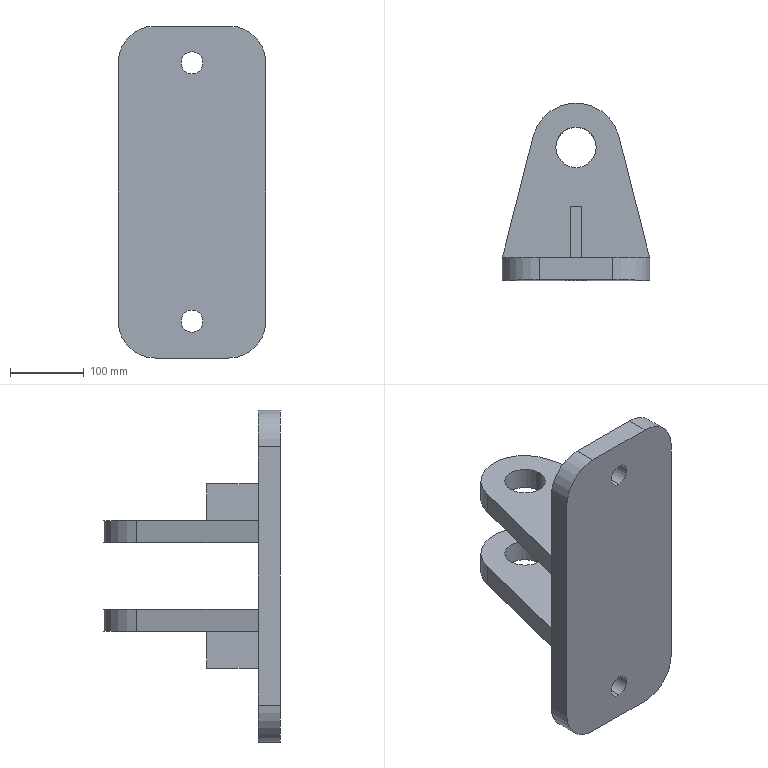Part | SolidWorks | features ICE 3, Extrusion 1, Fillet 1, MirrorPattern 1 | 1 solid | 38 faces | box 200 x 240 x 450 mm | volume 4353229 mm3 | plane 24 | cylinder 14 | commonest cylinder face diameters 30 x4 55 x4 100 x4 120 x2
STEP:
#1=CARTESIAN_POINT('',(0.,30.,160.));
#2=VERTEX_POINT('',#1);
#3=CARTESIAN_POINT('',(0.,30.,190.));
#4=VERTEX_POINT('',#3);
#5=CARTESIAN_POINT('',(0.,30.,175.));
#6=DIRECTION('',(0.,1.,0.));
#7=DIRECTION('',(0.,0.,-1.));
#8=AXIS2_PLACEMENT_3D('',#5,#6,#7);
#9=CIRCLE('',#8,15.);
#10=EDGE_CURVE('',#2,#4,#9,.T.);
#11=ORIENTED_EDGE('',*,*,#10,.T.);
#12=CARTESIAN_POINT('',(0.,0.,190.));
#13=VERTEX_POINT('',#12);
#14=CARTESIAN_POINT('',(0.,522.443,190.));
#15=DIRECTION('',(0.,-1.,0.));
#16=VECTOR('',#15,1000.);
#17=LINE('',#14,#16);
#18=EDGE_CURVE('',#4,#13,#17,.T.);
#19=ORIENTED_EDGE('',*,*,#18,.T.);
#20=CARTESIAN_POINT('',(0.,0.,160.));
#21=VERTEX_POINT('',#20);
#22=CARTESIAN_POINT('',(0.,0.,175.));
#23=DIRECTION('',(0.,-1.,0.));
#24=DIRECTION('',(0.,0.,1.));
#25=AXIS2_PLACEMENT_3D('',#22,#23,#24);
#26=CIRCLE('',#25,15.);
#27=EDGE_CURVE('',#13,#21,#26,.T.);
#28=ORIENTED_EDGE('',*,*,#27,.T.);
#29=CARTESIAN_POINT('',(0.,522.443,160.));
#30=DIRECTION('',(0.,-1.,0.));
#31=VECTOR('',#30,1000.);
#32=LINE('',#29,#31);
#33=EDGE_CURVE('',#2,#21,#32,.T.);
#34=ORIENTED_EDGE('',*,*,#33,.F.);
#35=EDGE_LOOP('',(#11,#19,#28,#34));
#36=FACE_OUTER_BOUND('',#35,.T.);
#37=CARTESIAN_POINT('',(0.,522.443,175.));
#38=DIRECTION('',(0.,-1.,0.));
#39=DIRECTION('',(0.,0.,-1.));
#40=AXIS2_PLACEMENT_3D('',#37,#38,#39);
#41=CYLINDRICAL_SURFACE('',#40,15.);
#42=ADVANCED_FACE('',(#36),#41,.F.);
#43=CARTESIAN_POINT('',(0.,30.,-190.));
#44=VERTEX_POINT('',#43);
#45=CARTESIAN_POINT('',(0.,30.,-160.));
#46=VERTEX_POINT('',#45);
#47=CARTESIAN_POINT('',(0.,30.,-175.));
#48=DIRECTION('',(0.,1.,0.));
#49=DIRECTION('',(0.,0.,-1.));
#50=AXIS2_PLACEMENT_3D('',#47,#48,#49);
#51=CIRCLE('',#50,15.);
#52=EDGE_CURVE('',#44,#46,#51,.T.);
#53=ORIENTED_EDGE('',*,*,#52,.T.);
#54=CARTESIAN_POINT('',(0.,0.,-160.));
#55=VERTEX_POINT('',#54);
#56=CARTESIAN_POINT('',(0.,522.443,-160.));
#57=DIRECTION('',(0.,-1.,0.));
#58=VECTOR('',#57,1000.);
#59=LINE('',#56,#58);
#60=EDGE_CURVE('',#46,#55,#59,.T.);
#61=ORIENTED_EDGE('',*,*,#60,.T.);
#62=CARTESIAN_POINT('',(0.,0.,-190.));
#63=VERTEX_POINT('',#62);
#64=CARTESIAN_POINT('',(0.,0.,-175.));
#65=DIRECTION('',(0.,-1.,0.));
#66=DIRECTION('',(0.,0.,-1.));
#67=AXIS2_PLACEMENT_3D('',#64,#65,#66);
#68=CIRCLE('',#67,15.);
#69=EDGE_CURVE('',#55,#63,#68,.T.);
#70=ORIENTED_EDGE('',*,*,#69,.T.);
#71=CARTESIAN_POINT('',(0.,522.443,-190.));
#72=DIRECTION('',(0.,-1.,0.));
#73=VECTOR('',#72,1000.);
#74=LINE('',#71,#73);
#75=EDGE_CURVE('',#44,#63,#74,.T.);
#76=ORIENTED_EDGE('',*,*,#75,.F.);
#77=EDGE_LOOP('',(#53,#61,#70,#76));
#78=FACE_OUTER_BOUND('',#77,.T.);
#79=CARTESIAN_POINT('',(0.,522.443,-175.));
#80=DIRECTION('',(0.,-1.,0.));
#81=DIRECTION('',(0.,0.,-1.));
#82=AXIS2_PLACEMENT_3D('',#79,#80,#81);
#83=CYLINDRICAL_SURFACE('',#82,15.);
#84=ADVANCED_FACE('',(#78),#83,.F.);
#85=CARTESIAN_POINT('',(-27.5,180.,-45.));
#86=VERTEX_POINT('',#85);
#87=CARTESIAN_POINT('',(27.5,180.,-45.));
#88=VERTEX_POINT('',#87);
#89=CARTESIAN_POINT('',(0.,180.,-45.));
#90=DIRECTION('',(0.,0.,1.));
#91=DIRECTION('',(1.,0.,0.));
#92=AXIS2_PLACEMENT_3D('',#89,#90,#91);
#93=CIRCLE('',#92,27.5);
#94=EDGE_CURVE('',#86,#88,#93,.T.);
#95=ORIENTED_EDGE('',*,*,#94,.T.);
#96=CARTESIAN_POINT('',(27.5,180.,-75.));
#97=VERTEX_POINT('',#96);
#98=CARTESIAN_POINT('',(27.5,180.,-45.));
#99=DIRECTION('',(0.,0.,-1.));
#100=VECTOR('',#99,1000.);
#101=LINE('',#98,#100);
#102=EDGE_CURVE('',#88,#97,#101,.T.);
#103=ORIENTED_EDGE('',*,*,#102,.T.);
#104=CARTESIAN_POINT('',(-27.5,180.,-75.));
#105=VERTEX_POINT('',#104);
#106=CARTESIAN_POINT('',(0.,180.,-75.));
#107=DIRECTION('',(0.,0.,1.));
#108=DIRECTION('',(1.,0.,0.));
#109=AXIS2_PLACEMENT_3D('',#106,#107,#108);
#110=CIRCLE('',#109,27.5);
#111=EDGE_CURVE('',#105,#97,#110,.T.);
#112=ORIENTED_EDGE('',*,*,#111,.F.);
#113=CARTESIAN_POINT('',(-27.5,180.,-45.));
#114=DIRECTION('',(0.,0.,-1.));
#115=VECTOR('',#114,1000.);
#116=LINE('',#113,#115);
#117=EDGE_CURVE('',#86,#105,#116,.T.);
#118=ORIENTED_EDGE('',*,*,#117,.F.);
#119=EDGE_LOOP('',(#95,#103,#112,#118));
#120=FACE_OUTER_BOUND('',#119,.T.);
#121=CARTESIAN_POINT('',(0.,180.,-45.));
#122=DIRECTION('',(0.,0.,-1.));
#123=DIRECTION('',(-1.,0.,0.));
#124=AXIS2_PLACEMENT_3D('',#121,#122,#123);
#125=CYLINDRICAL_SURFACE('',#124,27.5);
#126=ADVANCED_FACE('',(#120),#125,.F.);
#127=CARTESIAN_POINT('',(-27.5,180.,45.));
#128=VERTEX_POINT('',#127);
#129=CARTESIAN_POINT('',(27.5,180.,45.));
#130=VERTEX_POINT('',#129);
#131=CARTESIAN_POINT('',(0.,180.,45.));
#132=DIRECTION('',(0.,0.,1.));
#133=DIRECTION('',(1.,0.,0.));
#134=AXIS2_PLACEMENT_3D('',#131,#132,#133);
#135=CIRCLE('',#134,27.5);
#136=EDGE_CURVE('',#128,#130,#135,.T.);
#137=ORIENTED_EDGE('',*,*,#136,.F.);
#138=CARTESIAN_POINT('',(-27.5,180.,75.));
#139=VERTEX_POINT('',#138);
#140=CARTESIAN_POINT('',(-27.5,180.,45.));
#141=DIRECTION('',(0.,0.,1.));
#142=VECTOR('',#141,1000.);
#143=LINE('',#140,#142);
#144=EDGE_CURVE('',#128,#139,#143,.T.);
#145=ORIENTED_EDGE('',*,*,#144,.T.);
#146=CARTESIAN_POINT('',(27.5,180.,75.));
#147=VERTEX_POINT('',#146);
#148=CARTESIAN_POINT('',(0.,180.,75.));
#149=DIRECTION('',(0.,0.,1.));
#150=DIRECTION('',(1.,0.,0.));
#151=AXIS2_PLACEMENT_3D('',#148,#149,#150);
#152=CIRCLE('',#151,27.5);
#153=EDGE_CURVE('',#139,#147,#152,.T.);
#154=ORIENTED_EDGE('',*,*,#153,.T.);
#155=CARTESIAN_POINT('',(27.5,180.,45.));
#156=DIRECTION('',(0.,0.,1.));
#157=VECTOR('',#156,1000.);
#158=LINE('',#155,#157);
#159=EDGE_CURVE('',#130,#147,#158,.T.);
#160=ORIENTED_EDGE('',*,*,#159,.F.);
#161=EDGE_LOOP('',(#137,#145,#154,#160));
#162=FACE_OUTER_BOUND('',#161,.T.);
#163=CARTESIAN_POINT('',(0.,180.,45.));
#164=DIRECTION('',(0.,0.,1.));
#165=DIRECTION('',(1.,0.,0.));
#166=AXIS2_PLACEMENT_3D('',#163,#164,#165);
#167=CYLINDRICAL_SURFACE('',#166,27.5);
#168=ADVANCED_FACE('',(#162),#167,.F.);
#169=CARTESIAN_POINT('',(0.,180.,75.));
#170=DIRECTION('',(0.,0.,1.));
#171=DIRECTION('',(1.,0.,0.));
#172=AXIS2_PLACEMENT_3D('',#169,#170,#171);
#173=CIRCLE('',#172,27.5);
#174=EDGE_CURVE('',#147,#139,#173,.T.);
#175=ORIENTED_EDGE('',*,*,#174,.F.);
#176=ORIENTED_EDGE('',*,*,#153,.F.);
#177=EDGE_LOOP('',(#175,#176));
#178=FACE_BOUND('',#177,.T.);
#179=CARTESIAN_POINT('',(100.,30.,75.));
#180=VERTEX_POINT('',#179);
#181=CARTESIAN_POINT('',(7.5,30.,75.));
#182=VERTEX_POINT('',#181);
#183=CARTESIAN_POINT('',(-100.,30.,75.));
#184=DIRECTION('',(-1.,0.,0.));
#185=VECTOR('',#184,1000.);
#186=LINE('',#183,#185);
#187=EDGE_CURVE('',#180,#182,#186,.T.);
#188=ORIENTED_EDGE('',*,*,#187,.F.);
#189=CARTESIAN_POINT('',(58.154,194.769,75.));
#190=VERTEX_POINT('',#189);
#191=CARTESIAN_POINT('',(58.154,194.769,75.));
#192=DIRECTION('',(-0.2462,0.9692,0.));
#193=VECTOR('',#192,1000.);
#194=LINE('',#191,#193);
#195=EDGE_CURVE('',#180,#190,#194,.T.);
#196=ORIENTED_EDGE('',*,*,#195,.T.);
#197=CARTESIAN_POINT('',(-58.154,194.769,75.));
#198=VERTEX_POINT('',#197);
#199=CARTESIAN_POINT('',(0.,180.,75.));
#200=DIRECTION('',(0.,0.,1.));
#201=DIRECTION('',(1.,0.,0.));
#202=AXIS2_PLACEMENT_3D('',#199,#200,#201);
#203=CIRCLE('',#202,60.);
#204=EDGE_CURVE('',#190,#198,#203,.T.);
#205=ORIENTED_EDGE('',*,*,#204,.T.);
#206=CARTESIAN_POINT('',(-100.,30.,75.));
#207=VERTEX_POINT('',#206);
#208=CARTESIAN_POINT('',(-58.154,194.769,75.));
#209=DIRECTION('',(-0.2462,-0.9692,0.));
#210=VECTOR('',#209,1000.);
#211=LINE('',#208,#210);
#212=EDGE_CURVE('',#198,#207,#211,.T.);
#213=ORIENTED_EDGE('',*,*,#212,.T.);
#214=CARTESIAN_POINT('',(-7.5,30.,75.));
#215=VERTEX_POINT('',#214);
#216=CARTESIAN_POINT('',(-100.,30.,75.));
#217=DIRECTION('',(-1.,0.,0.));
#218=VECTOR('',#217,1000.);
#219=LINE('',#216,#218);
#220=EDGE_CURVE('',#215,#207,#219,.T.);
#221=ORIENTED_EDGE('',*,*,#220,.F.);
#222=CARTESIAN_POINT('',(-7.5,100.,75.));
#223=VERTEX_POINT('',#222);
#224=CARTESIAN_POINT('',(-7.5,100.,75.));
#225=DIRECTION('',(0.,-1.,0.));
#226=VECTOR('',#225,1000.);
#227=LINE('',#224,#226);
#228=EDGE_CURVE('',#223,#215,#227,.T.);
#229=ORIENTED_EDGE('',*,*,#228,.F.);
#230=CARTESIAN_POINT('',(7.5,100.,75.));
#231=VERTEX_POINT('',#230);
#232=CARTESIAN_POINT('',(-7.5,100.,75.));
#233=DIRECTION('',(-1.,0.,0.));
#234=VECTOR('',#233,1000.);
#235=LINE('',#232,#234);
#236=EDGE_CURVE('',#231,#223,#235,.T.);
#237=ORIENTED_EDGE('',*,*,#236,.F.);
#238=CARTESIAN_POINT('',(7.5,100.,75.));
#239=DIRECTION('',(0.,1.,0.));
#240=VECTOR('',#239,1000.);
#241=LINE('',#238,#240);
#242=EDGE_CURVE('',#182,#231,#241,.T.);
#243=ORIENTED_EDGE('',*,*,#242,.F.);
#244=EDGE_LOOP('',(#188,#196,#205,#213,#221,#229,#237,#243));
#245=FACE_OUTER_BOUND('',#244,.T.);
#246=CARTESIAN_POINT('',(-100.,30.,75.));
#247=DIRECTION('',(0.,0.,-1.));
#248=DIRECTION('',(-1.,0.,0.));
#249=AXIS2_PLACEMENT_3D('',#246,#247,#248);
#250=PLANE('',#249);
#251=ADVANCED_FACE('',(#178,#245),#250,.F.);
#252=ORIENTED_EDGE('',*,*,#111,.T.);
#253=CARTESIAN_POINT('',(0.,180.,-75.));
#254=DIRECTION('',(0.,0.,1.));
#255=DIRECTION('',(1.,0.,0.));
#256=AXIS2_PLACEMENT_3D('',#253,#254,#255);
#257=CIRCLE('',#256,27.5);
#258=EDGE_CURVE('',#97,#105,#257,.T.);
#259=ORIENTED_EDGE('',*,*,#258,.T.);
#260=EDGE_LOOP('',(#252,#259));
#261=FACE_BOUND('',#260,.T.);
#262=CARTESIAN_POINT('',(-100.,30.,-75.));
#263=VERTEX_POINT('',#262);
#264=CARTESIAN_POINT('',(-7.5,30.,-75.));
#265=VERTEX_POINT('',#264);
#266=CARTESIAN_POINT('',(-100.,30.,-75.));
#267=DIRECTION('',(1.,0.,0.));
#268=VECTOR('',#267,1000.);
#269=LINE('',#266,#268);
#270=EDGE_CURVE('',#263,#265,#269,.T.);
#271=ORIENTED_EDGE('',*,*,#270,.F.);
#272=CARTESIAN_POINT('',(-58.154,194.769,-75.));
#273=VERTEX_POINT('',#272);
#274=CARTESIAN_POINT('',(-58.154,194.769,-75.));
#275=DIRECTION('',(-0.2462,-0.9692,0.));
#276=VECTOR('',#275,1000.);
#277=LINE('',#274,#276);
#278=EDGE_CURVE('',#273,#263,#277,.T.);
#279=ORIENTED_EDGE('',*,*,#278,.F.);
#280=CARTESIAN_POINT('',(58.154,194.769,-75.));
#281=VERTEX_POINT('',#280);
#282=CARTESIAN_POINT('',(0.,180.,-75.));
#283=DIRECTION('',(0.,0.,1.));
#284=DIRECTION('',(1.,0.,0.));
#285=AXIS2_PLACEMENT_3D('',#282,#283,#284);
#286=CIRCLE('',#285,60.);
#287=EDGE_CURVE('',#281,#273,#286,.T.);
#288=ORIENTED_EDGE('',*,*,#287,.F.);
#289=CARTESIAN_POINT('',(100.,30.,-75.));
#290=VERTEX_POINT('',#289);
#291=CARTESIAN_POINT('',(58.154,194.769,-75.));
#292=DIRECTION('',(-0.2462,0.9692,0.));
#293=VECTOR('',#292,1000.);
#294=LINE('',#291,#293);
#295=EDGE_CURVE('',#290,#281,#294,.T.);
#296=ORIENTED_EDGE('',*,*,#295,.F.);
#297=CARTESIAN_POINT('',(7.5,30.,-75.));
#298=VERTEX_POINT('',#297);
#299=CARTESIAN_POINT('',(-100.,30.,-75.));
#300=DIRECTION('',(1.,0.,0.));
#301=VECTOR('',#300,1000.);
#302=LINE('',#299,#301);
#303=EDGE_CURVE('',#298,#290,#302,.T.);
#304=ORIENTED_EDGE('',*,*,#303,.F.);
#305=CARTESIAN_POINT('',(7.5,100.,-75.));
#306=VERTEX_POINT('',#305);
#307=CARTESIAN_POINT('',(7.5,100.,-75.));
#308=DIRECTION('',(0.,1.,0.));
#309=VECTOR('',#308,1000.);
#310=LINE('',#307,#309);
#311=EDGE_CURVE('',#298,#306,#310,.T.);
#312=ORIENTED_EDGE('',*,*,#311,.T.);
#313=CARTESIAN_POINT('',(-7.5,100.,-75.));
#314=VERTEX_POINT('',#313);
#315=CARTESIAN_POINT('',(-7.5,100.,-75.));
#316=DIRECTION('',(-1.,0.,0.));
#317=VECTOR('',#316,1000.);
#318=LINE('',#315,#317);
#319=EDGE_CURVE('',#306,#314,#318,.T.);
#320=ORIENTED_EDGE('',*,*,#319,.T.);
#321=CARTESIAN_POINT('',(-7.5,100.,-75.));
#322=DIRECTION('',(0.,-1.,0.));
#323=VECTOR('',#322,1000.);
#324=LINE('',#321,#323);
#325=EDGE_CURVE('',#314,#265,#324,.T.);
#326=ORIENTED_EDGE('',*,*,#325,.T.);
#327=EDGE_LOOP('',(#271,#279,#288,#296,#304,#312,#320,#326));
#328=FACE_OUTER_BOUND('',#327,.T.);
#329=CARTESIAN_POINT('',(-100.,30.,-75.));
#330=DIRECTION('',(0.,0.,1.));
#331=DIRECTION('',(1.,0.,0.));
#332=AXIS2_PLACEMENT_3D('',#329,#330,#331);
#333=PLANE('',#332);
#334=ADVANCED_FACE('',(#261,#328),#333,.F.);
#335=CARTESIAN_POINT('',(7.5,30.,125.));
#336=VERTEX_POINT('',#335);
#337=CARTESIAN_POINT('',(7.5,30.,125.));
#338=DIRECTION('',(0.,0.,1.));
#339=VECTOR('',#338,1000.);
#340=LINE('',#337,#339);
#341=EDGE_CURVE('',#182,#336,#340,.T.);
#342=ORIENTED_EDGE('',*,*,#341,.F.);
#343=ORIENTED_EDGE('',*,*,#242,.T.);
#344=CARTESIAN_POINT('',(7.5,100.,125.));
#345=VERTEX_POINT('',#344);
#346=CARTESIAN_POINT('',(7.5,100.,125.));
#347=DIRECTION('',(0.,0.,-1.));
#348=VECTOR('',#347,1000.);
#349=LINE('',#346,#348);
#350=EDGE_CURVE('',#345,#231,#349,.T.);
#351=ORIENTED_EDGE('',*,*,#350,.F.);
#352=CARTESIAN_POINT('',(7.5,100.,125.));
#353=DIRECTION('',(0.,1.,0.));
#354=VECTOR('',#353,1000.);
#355=LINE('',#352,#354);
#356=EDGE_CURVE('',#336,#345,#355,.T.);
#357=ORIENTED_EDGE('',*,*,#356,.F.);
#358=EDGE_LOOP('',(#342,#343,#351,#357));
#359=FACE_OUTER_BOUND('',#358,.T.);
#360=CARTESIAN_POINT('',(7.5,100.,125.));
#361=DIRECTION('',(-1.,0.,0.));
#362=DIRECTION('',(0.,-1.,0.));
#363=AXIS2_PLACEMENT_3D('',#360,#361,#362);
#364=PLANE('',#363);
#365=ADVANCED_FACE('',(#359),#364,.F.);
#366=CARTESIAN_POINT('',(-7.5,30.,125.));
#367=VERTEX_POINT('',#366);
#368=CARTESIAN_POINT('',(-7.5,30.,125.));
#369=DIRECTION('',(0.,0.,-1.));
#370=VECTOR('',#369,1000.);
#371=LINE('',#368,#370);
#372=EDGE_CURVE('',#367,#215,#371,.T.);
#373=ORIENTED_EDGE('',*,*,#372,.F.);
#374=CARTESIAN_POINT('',(-7.5,100.,125.));
#375=VERTEX_POINT('',#374);
#376=CARTESIAN_POINT('',(-7.5,100.,125.));
#377=DIRECTION('',(0.,-1.,0.));
#378=VECTOR('',#377,1000.);
#379=LINE('',#376,#378);
#380=EDGE_CURVE('',#375,#367,#379,.T.);
#381=ORIENTED_EDGE('',*,*,#380,.F.);
#382=CARTESIAN_POINT('',(-7.5,100.,125.));
#383=DIRECTION('',(0.,0.,-1.));
#384=VECTOR('',#383,1000.);
#385=LINE('',#382,#384);
#386=EDGE_CURVE('',#375,#223,#385,.T.);
#387=ORIENTED_EDGE('',*,*,#386,.T.);
#388=ORIENTED_EDGE('',*,*,#228,.T.);
#389=EDGE_LOOP('',(#373,#381,#387,#388));
#390=FACE_OUTER_BOUND('',#389,.T.);
#391=CARTESIAN_POINT('',(-7.5,100.,125.));
#392=DIRECTION('',(1.,0.,0.));
#393=DIRECTION('',(0.,1.,0.));
#394=AXIS2_PLACEMENT_3D('',#391,#392,#393);
#395=PLANE('',#394);
#396=ADVANCED_FACE('',(#390),#395,.F.);
#397=ORIENTED_EDGE('',*,*,#380,.T.);
#398=CARTESIAN_POINT('',(0.,30.,125.));
#399=DIRECTION('',(1.,0.,0.));
#400=VECTOR('',#399,1000.);
#401=LINE('',#398,#400);
#402=EDGE_CURVE('',#367,#336,#401,.T.);
#403=ORIENTED_EDGE('',*,*,#402,.T.);
#404=ORIENTED_EDGE('',*,*,#356,.T.);
#405=CARTESIAN_POINT('',(-7.5,100.,125.));
#406=DIRECTION('',(-1.,0.,0.));
#407=VECTOR('',#406,1000.);
#408=LINE('',#405,#407);
#409=EDGE_CURVE('',#345,#375,#408,.T.);
#410=ORIENTED_EDGE('',*,*,#409,.T.);
#411=EDGE_LOOP('',(#397,#403,#404,#410));
#412=FACE_OUTER_BOUND('',#411,.T.);
#413=CARTESIAN_POINT('',(0.,0.,125.));
#414=DIRECTION('',(0.,0.,1.));
#415=DIRECTION('',(1.,0.,0.));
#416=AXIS2_PLACEMENT_3D('',#413,#414,#415);
#417=PLANE('',#416);
#418=ADVANCED_FACE('',(#412),#417,.T.);
#419=ORIENTED_EDGE('',*,*,#311,.F.);
#420=CARTESIAN_POINT('',(7.5,30.,-125.));
#421=VERTEX_POINT('',#420);
#422=CARTESIAN_POINT('',(7.5,30.,-125.));
#423=DIRECTION('',(0.,0.,-1.));
#424=VECTOR('',#423,1000.);
#425=LINE('',#422,#424);
#426=EDGE_CURVE('',#298,#421,#425,.T.);
#427=ORIENTED_EDGE('',*,*,#426,.T.);
#428=CARTESIAN_POINT('',(7.5,100.,-125.));
#429=VERTEX_POINT('',#428);
#430=CARTESIAN_POINT('',(7.5,100.,-125.));
#431=DIRECTION('',(0.,1.,0.));
#432=VECTOR('',#431,1000.);
#433=LINE('',#430,#432);
#434=EDGE_CURVE('',#421,#429,#433,.T.);
#435=ORIENTED_EDGE('',*,*,#434,.T.);
#436=CARTESIAN_POINT('',(7.5,100.,-125.));
#437=DIRECTION('',(0.,0.,1.));
#438=VECTOR('',#437,1000.);
#439=LINE('',#436,#438);
#440=EDGE_CURVE('',#429,#306,#439,.T.);
#441=ORIENTED_EDGE('',*,*,#440,.T.);
#442=EDGE_LOOP('',(#419,#427,#435,#441));
#443=FACE_OUTER_BOUND('',#442,.T.);
#444=CARTESIAN_POINT('',(7.5,100.,-125.));
#445=DIRECTION('',(1.,0.,0.));
#446=DIRECTION('',(0.,1.,0.));
#447=AXIS2_PLACEMENT_3D('',#444,#445,#446);
#448=PLANE('',#447);
#449=ADVANCED_FACE('',(#443),#448,.T.);
#450=CARTESIAN_POINT('',(-7.5,100.,-125.));
#451=VERTEX_POINT('',#450);
#452=CARTESIAN_POINT('',(-7.5,30.,-125.));
#453=VERTEX_POINT('',#452);
#454=CARTESIAN_POINT('',(-7.5,100.,-125.));
#455=DIRECTION('',(0.,-1.,0.));
#456=VECTOR('',#455,1000.);
#457=LINE('',#454,#456);
#458=EDGE_CURVE('',#451,#453,#457,.T.);
#459=ORIENTED_EDGE('',*,*,#458,.T.);
#460=CARTESIAN_POINT('',(-7.5,30.,-125.));
#461=DIRECTION('',(0.,0.,1.));
#462=VECTOR('',#461,1000.);
#463=LINE('',#460,#462);
#464=EDGE_CURVE('',#453,#265,#463,.T.);
#465=ORIENTED_EDGE('',*,*,#464,.T.);
#466=ORIENTED_EDGE('',*,*,#325,.F.);
#467=CARTESIAN_POINT('',(-7.5,100.,-125.));
#468=DIRECTION('',(0.,0.,1.));
#469=VECTOR('',#468,1000.);
#470=LINE('',#467,#469);
#471=EDGE_CURVE('',#451,#314,#470,.T.);
#472=ORIENTED_EDGE('',*,*,#471,.F.);
#473=EDGE_LOOP('',(#459,#465,#466,#472));
#474=FACE_OUTER_BOUND('',#473,.T.);
#475=CARTESIAN_POINT('',(-7.5,100.,-125.));
#476=DIRECTION('',(-1.,0.,0.));
#477=DIRECTION('',(0.,-1.,0.));
#478=AXIS2_PLACEMENT_3D('',#475,#476,#477);
#479=PLANE('',#478);
#480=ADVANCED_FACE('',(#474),#479,.T.);
#481=ORIENTED_EDGE('',*,*,#434,.F.);
#482=CARTESIAN_POINT('',(0.,30.,-125.));
#483=DIRECTION('',(-1.,0.,0.));
#484=VECTOR('',#483,1000.);
#485=LINE('',#482,#484);
#486=EDGE_CURVE('',#421,#453,#485,.T.);
#487=ORIENTED_EDGE('',*,*,#486,.T.);
#488=ORIENTED_EDGE('',*,*,#458,.F.);
#489=CARTESIAN_POINT('',(-7.5,100.,-125.));
#490=DIRECTION('',(-1.,0.,0.));
#491=VECTOR('',#490,1000.);
#492=LINE('',#489,#491);
#493=EDGE_CURVE('',#429,#451,#492,.T.);
#494=ORIENTED_EDGE('',*,*,#493,.F.);
#495=EDGE_LOOP('',(#481,#487,#488,#494));
#496=FACE_OUTER_BOUND('',#495,.T.);
#497=CARTESIAN_POINT('',(0.,0.,-125.));
#498=DIRECTION('',(0.,0.,-1.));
#499=DIRECTION('',(1.,0.,0.));
#500=AXIS2_PLACEMENT_3D('',#497,#498,#499);
#501=PLANE('',#500);
#502=ADVANCED_FACE('',(#496),#501,.T.);
#503=CARTESIAN_POINT('',(-100.,30.,-45.));
#504=VERTEX_POINT('',#503);
#505=CARTESIAN_POINT('',(100.,30.,-45.));
#506=VERTEX_POINT('',#505);
#507=CARTESIAN_POINT('',(-100.,30.,-45.));
#508=DIRECTION('',(1.,0.,0.));
#509=VECTOR('',#508,1000.);
#510=LINE('',#507,#509);
#511=EDGE_CURVE('',#504,#506,#510,.T.);
#512=ORIENTED_EDGE('',*,*,#511,.F.);
#513=CARTESIAN_POINT('',(-100.,30.,45.));
#514=VERTEX_POINT('',#513);
#515=CARTESIAN_POINT('',(-100.,30.,75.));
#516=DIRECTION('',(0.,0.,1.));
#517=VECTOR('',#516,1000.);
#518=LINE('',#515,#517);
#519=EDGE_CURVE('',#504,#514,#518,.T.);
#520=ORIENTED_EDGE('',*,*,#519,.T.);
#521=CARTESIAN_POINT('',(100.,30.,45.));
#522=VERTEX_POINT('',#521);
#523=CARTESIAN_POINT('',(-100.,30.,45.));
#524=DIRECTION('',(1.,0.,0.));
#525=VECTOR('',#524,1000.);
#526=LINE('',#523,#525);
#527=EDGE_CURVE('',#514,#522,#526,.T.);
#528=ORIENTED_EDGE('',*,*,#527,.T.);
#529=CARTESIAN_POINT('',(100.,30.,75.));
#530=DIRECTION('',(0.,0.,-1.));
#531=VECTOR('',#530,1000.);
#532=LINE('',#529,#531);
#533=EDGE_CURVE('',#522,#506,#532,.T.);
#534=ORIENTED_EDGE('',*,*,#533,.T.);
#535=EDGE_LOOP('',(#512,#520,#528,#534));
#536=FACE_OUTER_BOUND('',#535,.T.);
#537=CARTESIAN_POINT('',(0.,30.,0.));
#538=DIRECTION('',(0.,-1.,0.));
#539=DIRECTION('',(0.,0.,-1.));
#540=AXIS2_PLACEMENT_3D('',#537,#538,#539);
#541=PLANE('',#540);
#542=ADVANCED_FACE('',(#536),#541,.F.);
#543=CARTESIAN_POINT('',(100.,30.,175.));
#544=VERTEX_POINT('',#543);
#545=CARTESIAN_POINT('',(100.,30.,-225.));
#546=DIRECTION('',(0.,0.,-1.));
#547=VECTOR('',#546,1000.);
#548=LINE('',#545,#547);
#549=EDGE_CURVE('',#544,#180,#548,.T.);
#550=ORIENTED_EDGE('',*,*,#549,.F.);
#551=CARTESIAN_POINT('',(100.,0.,175.));
#552=VERTEX_POINT('',#551);
#553=CARTESIAN_POINT('',(100.,0.,175.));
#554=DIRECTION('',(0.,-1.,0.));
#555=VECTOR('',#554,1000.);
#556=LINE('',#553,#555);
#557=EDGE_CURVE('',#544,#552,#556,.T.);
#558=ORIENTED_EDGE('',*,*,#557,.T.);
#559=CARTESIAN_POINT('',(100.,0.,-175.));
#560=VERTEX_POINT('',#559);
#561=CARTESIAN_POINT('',(100.,0.,75.));
#562=DIRECTION('',(0.,0.,-1.));
#563=VECTOR('',#562,1000.);
#564=LINE('',#561,#563);
#565=EDGE_CURVE('',#552,#560,#564,.T.);
#566=ORIENTED_EDGE('',*,*,#565,.T.);
#567=CARTESIAN_POINT('',(100.,30.,-175.));
#568=VERTEX_POINT('',#567);
#569=CARTESIAN_POINT('',(100.,30.,-175.));
#570=DIRECTION('',(0.,1.,0.));
#571=VECTOR('',#570,1000.);
#572=LINE('',#569,#571);
#573=EDGE_CURVE('',#560,#568,#572,.T.);
#574=ORIENTED_EDGE('',*,*,#573,.T.);
#575=CARTESIAN_POINT('',(100.,30.,-225.));
#576=DIRECTION('',(0.,0.,-1.));
#577=VECTOR('',#576,1000.);
#578=LINE('',#575,#577);
#579=EDGE_CURVE('',#290,#568,#578,.T.);
#580=ORIENTED_EDGE('',*,*,#579,.F.);
#581=CARTESIAN_POINT('',(100.,30.,-45.));
#582=DIRECTION('',(0.,0.,-1.));
#583=VECTOR('',#582,1000.);
#584=LINE('',#581,#583);
#585=EDGE_CURVE('',#506,#290,#584,.T.);
#586=ORIENTED_EDGE('',*,*,#585,.F.);
#587=ORIENTED_EDGE('',*,*,#533,.F.);
#588=CARTESIAN_POINT('',(100.,30.,75.));
#589=DIRECTION('',(0.,0.,-1.));
#590=VECTOR('',#589,1000.);
#591=LINE('',#588,#590);
#592=EDGE_CURVE('',#180,#522,#591,.T.);
#593=ORIENTED_EDGE('',*,*,#592,.F.);
#594=EDGE_LOOP('',(#550,#558,#566,#574,#580,#586,#587,#593));
#595=FACE_OUTER_BOUND('',#594,.T.);
#596=CARTESIAN_POINT('',(100.,30.,75.));
#597=DIRECTION('',(-1.,0.,0.));
#598=DIRECTION('',(0.,0.,1.));
#599=AXIS2_PLACEMENT_3D('',#596,#597,#598);
#600=PLANE('',#599);
#601=ADVANCED_FACE('',(#595),#600,.F.);
#602=CARTESIAN_POINT('',(-100.,0.,-175.));
#603=VERTEX_POINT('',#602);
#604=CARTESIAN_POINT('',(-100.,0.,175.));
#605=VERTEX_POINT('',#604);
#606=CARTESIAN_POINT('',(-100.,0.,75.));
#607=DIRECTION('',(0.,0.,1.));
#608=VECTOR('',#607,1000.);
#609=LINE('',#606,#608);
#610=EDGE_CURVE('',#603,#605,#609,.T.);
#611=ORIENTED_EDGE('',*,*,#610,.T.);
#612=CARTESIAN_POINT('',(-100.,30.,175.));
#613=VERTEX_POINT('',#612);
#614=CARTESIAN_POINT('',(-100.,30.,175.));
#615=DIRECTION('',(0.,1.,0.));
#616=VECTOR('',#615,1000.);
#617=LINE('',#614,#616);
#618=EDGE_CURVE('',#605,#613,#617,.T.);
#619=ORIENTED_EDGE('',*,*,#618,.T.);
#620=CARTESIAN_POINT('',(-100.,30.,-225.));
#621=DIRECTION('',(0.,0.,1.));
#622=VECTOR('',#621,1000.);
#623=LINE('',#620,#622);
#624=EDGE_CURVE('',#207,#613,#623,.T.);
#625=ORIENTED_EDGE('',*,*,#624,.F.);
#626=CARTESIAN_POINT('',(-100.,30.,45.));
#627=DIRECTION('',(0.,0.,1.));
#628=VECTOR('',#627,1000.);
#629=LINE('',#626,#628);
#630=EDGE_CURVE('',#514,#207,#629,.T.);
#631=ORIENTED_EDGE('',*,*,#630,.F.);
#632=ORIENTED_EDGE('',*,*,#519,.F.);
#633=CARTESIAN_POINT('',(-100.,30.,75.));
#634=DIRECTION('',(0.,0.,1.));
#635=VECTOR('',#634,1000.);
#636=LINE('',#633,#635);
#637=EDGE_CURVE('',#263,#504,#636,.T.);
#638=ORIENTED_EDGE('',*,*,#637,.F.);
#639=CARTESIAN_POINT('',(-100.,30.,-175.));
#640=VERTEX_POINT('',#639);
#641=CARTESIAN_POINT('',(-100.,30.,-225.));
#642=DIRECTION('',(0.,0.,1.));
#643=VECTOR('',#642,1000.);
#644=LINE('',#641,#643);
#645=EDGE_CURVE('',#640,#263,#644,.T.);
#646=ORIENTED_EDGE('',*,*,#645,.F.);
#647=CARTESIAN_POINT('',(-100.,0.,-175.));
#648=DIRECTION('',(0.,-1.,0.));
#649=VECTOR('',#648,1000.);
#650=LINE('',#647,#649);
#651=EDGE_CURVE('',#640,#603,#650,.T.);
#652=ORIENTED_EDGE('',*,*,#651,.T.);
#653=EDGE_LOOP('',(#611,#619,#625,#631,#632,#638,#646,#652));
#654=FACE_OUTER_BOUND('',#653,.T.);
#655=CARTESIAN_POINT('',(-100.,30.,75.));
#656=DIRECTION('',(1.,0.,0.));
#657=DIRECTION('',(0.,0.,-1.));
#658=AXIS2_PLACEMENT_3D('',#655,#656,#657);
#659=PLANE('',#658);
#660=ADVANCED_FACE('',(#654),#659,.F.);
#661=ORIENTED_EDGE('',*,*,#565,.F.);
#662=CARTESIAN_POINT('',(50.,0.,225.));
#663=VERTEX_POINT('',#662);
#664=CARTESIAN_POINT('',(50.,0.,175.));
#665=DIRECTION('',(0.,-1.,0.));
#666=DIRECTION('',(0.,0.,-1.));
#667=AXIS2_PLACEMENT_3D('',#664,#665,#666);
#668=CIRCLE('',#667,50.);
#669=EDGE_CURVE('',#552,#663,#668,.T.);
#670=ORIENTED_EDGE('',*,*,#669,.T.);
#671=CARTESIAN_POINT('',(-50.,0.,225.));
#672=VERTEX_POINT('',#671);
#673=CARTESIAN_POINT('',(100.,0.,225.));
#674=DIRECTION('',(-1.,0.,0.));
#675=VECTOR('',#674,1000.);
#676=LINE('',#673,#675);
#677=EDGE_CURVE('',#663,#672,#676,.T.);
#678=ORIENTED_EDGE('',*,*,#677,.T.);
#679=CARTESIAN_POINT('',(-50.,0.,175.));
#680=DIRECTION('',(0.,-1.,0.));
#681=DIRECTION('',(0.,0.,-1.));
#682=AXIS2_PLACEMENT_3D('',#679,#680,#681);
#683=CIRCLE('',#682,50.);
#684=EDGE_CURVE('',#672,#605,#683,.T.);
#685=ORIENTED_EDGE('',*,*,#684,.T.);
#686=ORIENTED_EDGE('',*,*,#610,.F.);
#687=CARTESIAN_POINT('',(-50.,0.,-225.));
#688=VERTEX_POINT('',#687);
#689=CARTESIAN_POINT('',(-50.,0.,-175.));
#690=DIRECTION('',(0.,-1.,0.));
#691=DIRECTION('',(0.,0.,-1.));
#692=AXIS2_PLACEMENT_3D('',#689,#690,#691);
#693=CIRCLE('',#692,50.);
#694=EDGE_CURVE('',#603,#688,#693,.T.);
#695=ORIENTED_EDGE('',*,*,#694,.T.);
#696=CARTESIAN_POINT('',(50.,0.,-225.));
#697=VERTEX_POINT('',#696);
#698=CARTESIAN_POINT('',(100.,0.,-225.));
#699=DIRECTION('',(1.,0.,0.));
#700=VECTOR('',#699,1000.);
#701=LINE('',#698,#700);
#702=EDGE_CURVE('',#688,#697,#701,.T.);
#703=ORIENTED_EDGE('',*,*,#702,.T.);
#704=CARTESIAN_POINT('',(50.,0.,-175.));
#705=DIRECTION('',(0.,-1.,0.));
#706=DIRECTION('',(0.,0.,-1.));
#707=AXIS2_PLACEMENT_3D('',#704,#705,#706);
#708=CIRCLE('',#707,50.);
#709=EDGE_CURVE('',#697,#560,#708,.T.);
#710=ORIENTED_EDGE('',*,*,#709,.T.);
#711=EDGE_LOOP('',(#661,#670,#678,#685,#686,#695,#703,#710));
#712=FACE_OUTER_BOUND('',#711,.T.);
#713=CARTESIAN_POINT('',(0.,0.,-175.));
#714=DIRECTION('',(0.,-1.,0.));
#715=DIRECTION('',(0.,0.,-1.));
#716=AXIS2_PLACEMENT_3D('',#713,#714,#715);
#717=CIRCLE('',#716,15.);
#718=EDGE_CURVE('',#63,#55,#717,.T.);
#719=ORIENTED_EDGE('',*,*,#718,.F.);
#720=ORIENTED_EDGE('',*,*,#69,.F.);
#721=EDGE_LOOP('',(#719,#720));
#722=FACE_BOUND('',#721,.T.);
#723=CARTESIAN_POINT('',(0.,0.,175.));
#724=DIRECTION('',(0.,-1.,0.));
#725=DIRECTION('',(0.,0.,1.));
#726=AXIS2_PLACEMENT_3D('',#723,#724,#725);
#727=CIRCLE('',#726,15.);
#728=EDGE_CURVE('',#21,#13,#727,.T.);
#729=ORIENTED_EDGE('',*,*,#728,.F.);
#730=ORIENTED_EDGE('',*,*,#27,.F.);
#731=EDGE_LOOP('',(#729,#730));
#732=FACE_BOUND('',#731,.T.);
#733=CARTESIAN_POINT('',(0.,0.,0.));
#734=DIRECTION('',(0.,-1.,0.));
#735=DIRECTION('',(0.,0.,-1.));
#736=AXIS2_PLACEMENT_3D('',#733,#734,#735);
#737=PLANE('',#736);
#738=ADVANCED_FACE('',(#712,#722,#732),#737,.T.);
#739=ORIENTED_EDGE('',*,*,#204,.F.);
#740=CARTESIAN_POINT('',(58.154,194.769,45.));
#741=VERTEX_POINT('',#740);
#742=CARTESIAN_POINT('',(58.154,194.769,45.));
#743=DIRECTION('',(0.,0.,1.));
#744=VECTOR('',#743,1000.);
#745=LINE('',#742,#744);
#746=EDGE_CURVE('',#741,#190,#745,.T.);
#747=ORIENTED_EDGE('',*,*,#746,.F.);
#748=CARTESIAN_POINT('',(-58.154,194.769,45.));
#749=VERTEX_POINT('',#748);
#750=CARTESIAN_POINT('',(0.,180.,45.));
#751=DIRECTION('',(0.,0.,1.));
#752=DIRECTION('',(1.,0.,0.));
#753=AXIS2_PLACEMENT_3D('',#750,#751,#752);
#754=CIRCLE('',#753,60.);
#755=EDGE_CURVE('',#741,#749,#754,.T.);
#756=ORIENTED_EDGE('',*,*,#755,.T.);
#757=CARTESIAN_POINT('',(-58.154,194.769,45.));
#758=DIRECTION('',(0.,0.,1.));
#759=VECTOR('',#758,1000.);
#760=LINE('',#757,#759);
#761=EDGE_CURVE('',#749,#198,#760,.T.);
#762=ORIENTED_EDGE('',*,*,#761,.T.);
#763=EDGE_LOOP('',(#739,#747,#756,#762));
#764=FACE_OUTER_BOUND('',#763,.T.);
#765=CARTESIAN_POINT('',(0.,180.,45.));
#766=DIRECTION('',(0.,0.,1.));
#767=DIRECTION('',(1.,0.,0.));
#768=AXIS2_PLACEMENT_3D('',#765,#766,#767);
#769=CYLINDRICAL_SURFACE('',#768,60.);
#770=ADVANCED_FACE('',(#764),#769,.T.);
#771=ORIENTED_EDGE('',*,*,#195,.F.);
#772=ORIENTED_EDGE('',*,*,#592,.T.);
#773=CARTESIAN_POINT('',(58.154,194.769,45.));
#774=DIRECTION('',(-0.2462,0.9692,0.));
#775=VECTOR('',#774,1000.);
#776=LINE('',#773,#775);
#777=EDGE_CURVE('',#522,#741,#776,.T.);
#778=ORIENTED_EDGE('',*,*,#777,.T.);
#779=ORIENTED_EDGE('',*,*,#746,.T.);
#780=EDGE_LOOP('',(#771,#772,#778,#779));
#781=FACE_OUTER_BOUND('',#780,.T.);
#782=CARTESIAN_POINT('',(58.154,194.769,45.));
#783=DIRECTION('',(0.9692,0.2462,0.));
#784=DIRECTION('',(-0.2462,0.9692,0.));
#785=AXIS2_PLACEMENT_3D('',#782,#783,#784);
#786=PLANE('',#785);
#787=ADVANCED_FACE('',(#781),#786,.T.);
#788=ORIENTED_EDGE('',*,*,#212,.F.);
#789=ORIENTED_EDGE('',*,*,#761,.F.);
#790=CARTESIAN_POINT('',(-58.154,194.769,45.));
#791=DIRECTION('',(-0.2462,-0.9692,0.));
#792=VECTOR('',#791,1000.);
#793=LINE('',#790,#792);
#794=EDGE_CURVE('',#749,#514,#793,.T.);
#795=ORIENTED_EDGE('',*,*,#794,.T.);
#796=ORIENTED_EDGE('',*,*,#630,.T.);
#797=EDGE_LOOP('',(#788,#789,#795,#796));
#798=FACE_OUTER_BOUND('',#797,.T.);
#799=CARTESIAN_POINT('',(-58.154,194.769,45.));
#800=DIRECTION('',(-0.9692,0.2462,0.));
#801=DIRECTION('',(-0.2462,-0.9692,0.));
#802=AXIS2_PLACEMENT_3D('',#799,#800,#801);
#803=PLANE('',#802);
#804=ADVANCED_FACE('',(#798),#803,.T.);
#805=CARTESIAN_POINT('',(0.,180.,45.));
#806=DIRECTION('',(0.,0.,1.));
#807=DIRECTION('',(1.,0.,0.));
#808=AXIS2_PLACEMENT_3D('',#805,#806,#807);
#809=CIRCLE('',#808,27.5);
#810=EDGE_CURVE('',#130,#128,#809,.T.);
#811=ORIENTED_EDGE('',*,*,#810,.T.);
#812=ORIENTED_EDGE('',*,*,#136,.T.);
#813=EDGE_LOOP('',(#811,#812));
#814=FACE_BOUND('',#813,.T.);
#815=ORIENTED_EDGE('',*,*,#755,.F.);
#816=ORIENTED_EDGE('',*,*,#777,.F.);
#817=ORIENTED_EDGE('',*,*,#527,.F.);
#818=ORIENTED_EDGE('',*,*,#794,.F.);
#819=EDGE_LOOP('',(#815,#816,#817,#818));
#820=FACE_OUTER_BOUND('',#819,.T.);
#821=CARTESIAN_POINT('',(0.,180.,45.));
#822=DIRECTION('',(0.,0.,1.));
#823=DIRECTION('',(1.,0.,0.));
#824=AXIS2_PLACEMENT_3D('',#821,#822,#823);
#825=PLANE('',#824);
#826=ADVANCED_FACE('',(#814,#820),#825,.F.);
#827=ORIENTED_EDGE('',*,*,#144,.F.);
#828=ORIENTED_EDGE('',*,*,#810,.F.);
#829=ORIENTED_EDGE('',*,*,#159,.T.);
#830=ORIENTED_EDGE('',*,*,#174,.T.);
#831=EDGE_LOOP('',(#827,#828,#829,#830));
#832=FACE_OUTER_BOUND('',#831,.T.);
#833=CARTESIAN_POINT('',(0.,180.,45.));
#834=DIRECTION('',(0.,0.,1.));
#835=DIRECTION('',(1.,0.,0.));
#836=AXIS2_PLACEMENT_3D('',#833,#834,#835);
#837=CYLINDRICAL_SURFACE('',#836,27.5);
#838=ADVANCED_FACE('',(#832),#837,.F.);
#839=ORIENTED_EDGE('',*,*,#236,.T.);
#840=ORIENTED_EDGE('',*,*,#386,.F.);
#841=ORIENTED_EDGE('',*,*,#409,.F.);
#842=ORIENTED_EDGE('',*,*,#350,.T.);
#843=EDGE_LOOP('',(#839,#840,#841,#842));
#844=FACE_OUTER_BOUND('',#843,.T.);
#845=CARTESIAN_POINT('',(-7.5,100.,125.));
#846=DIRECTION('',(0.,-1.,0.));
#847=DIRECTION('',(0.,0.,-1.));
#848=AXIS2_PLACEMENT_3D('',#845,#846,#847);
#849=PLANE('',#848);
#850=ADVANCED_FACE('',(#844),#849,.F.);
#851=CARTESIAN_POINT('',(58.154,194.769,-45.));
#852=VERTEX_POINT('',#851);
#853=CARTESIAN_POINT('',(-58.154,194.769,-45.));
#854=VERTEX_POINT('',#853);
#855=CARTESIAN_POINT('',(0.,180.,-45.));
#856=DIRECTION('',(0.,0.,1.));
#857=DIRECTION('',(1.,0.,0.));
#858=AXIS2_PLACEMENT_3D('',#855,#856,#857);
#859=CIRCLE('',#858,60.);
#860=EDGE_CURVE('',#852,#854,#859,.T.);
#861=ORIENTED_EDGE('',*,*,#860,.T.);
#862=CARTESIAN_POINT('',(-58.154,194.769,-45.));
#863=DIRECTION('',(-0.2462,-0.9692,0.));
#864=VECTOR('',#863,1000.);
#865=LINE('',#862,#864);
#866=EDGE_CURVE('',#854,#504,#865,.T.);
#867=ORIENTED_EDGE('',*,*,#866,.T.);
#868=ORIENTED_EDGE('',*,*,#511,.T.);
#869=CARTESIAN_POINT('',(58.154,194.769,-45.));
#870=DIRECTION('',(-0.2462,0.9692,0.));
#871=VECTOR('',#870,1000.);
#872=LINE('',#869,#871);
#873=EDGE_CURVE('',#506,#852,#872,.T.);
#874=ORIENTED_EDGE('',*,*,#873,.T.);
#875=EDGE_LOOP('',(#861,#867,#868,#874));
#876=FACE_OUTER_BOUND('',#875,.T.);
#877=ORIENTED_EDGE('',*,*,#94,.F.);
#878=CARTESIAN_POINT('',(0.,180.,-45.));
#879=DIRECTION('',(0.,0.,1.));
#880=DIRECTION('',(1.,0.,0.));
#881=AXIS2_PLACEMENT_3D('',#878,#879,#880);
#882=CIRCLE('',#881,27.5);
#883=EDGE_CURVE('',#88,#86,#882,.T.);
#884=ORIENTED_EDGE('',*,*,#883,.F.);
#885=EDGE_LOOP('',(#877,#884));
#886=FACE_BOUND('',#885,.T.);
#887=CARTESIAN_POINT('',(0.,180.,-45.));
#888=DIRECTION('',(0.,0.,-1.));
#889=DIRECTION('',(1.,0.,0.));
#890=AXIS2_PLACEMENT_3D('',#887,#888,#889);
#891=PLANE('',#890);
#892=ADVANCED_FACE('',(#876,#886),#891,.F.);
#893=ORIENTED_EDGE('',*,*,#287,.T.);
#894=CARTESIAN_POINT('',(-58.154,194.769,-45.));
#895=DIRECTION('',(0.,0.,-1.));
#896=VECTOR('',#895,1000.);
#897=LINE('',#894,#896);
#898=EDGE_CURVE('',#854,#273,#897,.T.);
#899=ORIENTED_EDGE('',*,*,#898,.F.);
#900=ORIENTED_EDGE('',*,*,#860,.F.);
#901=CARTESIAN_POINT('',(58.154,194.769,-45.));
#902=DIRECTION('',(0.,0.,-1.));
#903=VECTOR('',#902,1000.);
#904=LINE('',#901,#903);
#905=EDGE_CURVE('',#852,#281,#904,.T.);
#906=ORIENTED_EDGE('',*,*,#905,.T.);
#907=EDGE_LOOP('',(#893,#899,#900,#906));
#908=FACE_OUTER_BOUND('',#907,.T.);
#909=CARTESIAN_POINT('',(0.,180.,-45.));
#910=DIRECTION('',(0.,0.,-1.));
#911=DIRECTION('',(-1.,0.,0.));
#912=AXIS2_PLACEMENT_3D('',#909,#910,#911);
#913=CYLINDRICAL_SURFACE('',#912,60.);
#914=ADVANCED_FACE('',(#908),#913,.T.);
#915=ORIENTED_EDGE('',*,*,#278,.T.);
#916=ORIENTED_EDGE('',*,*,#637,.T.);
#917=ORIENTED_EDGE('',*,*,#866,.F.);
#918=ORIENTED_EDGE('',*,*,#898,.T.);
#919=EDGE_LOOP('',(#915,#916,#917,#918));
#920=FACE_OUTER_BOUND('',#919,.T.);
#921=CARTESIAN_POINT('',(-58.154,194.769,-45.));
#922=DIRECTION('',(0.9692,-0.2462,0.));
#923=DIRECTION('',(0.2462,0.9692,0.));
#924=AXIS2_PLACEMENT_3D('',#921,#922,#923);
#925=PLANE('',#924);
#926=ADVANCED_FACE('',(#920),#925,.F.);
#927=ORIENTED_EDGE('',*,*,#295,.T.);
#928=ORIENTED_EDGE('',*,*,#905,.F.);
#929=ORIENTED_EDGE('',*,*,#873,.F.);
#930=ORIENTED_EDGE('',*,*,#585,.T.);
#931=EDGE_LOOP('',(#927,#928,#929,#930));
#932=FACE_OUTER_BOUND('',#931,.T.);
#933=CARTESIAN_POINT('',(58.154,194.769,-45.));
#934=DIRECTION('',(-0.9692,-0.2462,0.));
#935=DIRECTION('',(0.2462,-0.9692,0.));
#936=AXIS2_PLACEMENT_3D('',#933,#934,#935);
#937=PLANE('',#936);
#938=ADVANCED_FACE('',(#932),#937,.F.);
#939=ORIENTED_EDGE('',*,*,#102,.F.);
#940=ORIENTED_EDGE('',*,*,#883,.T.);
#941=ORIENTED_EDGE('',*,*,#117,.T.);
#942=ORIENTED_EDGE('',*,*,#258,.F.);
#943=EDGE_LOOP('',(#939,#940,#941,#942));
#944=FACE_OUTER_BOUND('',#943,.T.);
#945=CARTESIAN_POINT('',(0.,180.,-45.));
#946=DIRECTION('',(0.,0.,-1.));
#947=DIRECTION('',(-1.,0.,0.));
#948=AXIS2_PLACEMENT_3D('',#945,#946,#947);
#949=CYLINDRICAL_SURFACE('',#948,27.5);
#950=ADVANCED_FACE('',(#944),#949,.F.);
#951=ORIENTED_EDGE('',*,*,#319,.F.);
#952=ORIENTED_EDGE('',*,*,#440,.F.);
#953=ORIENTED_EDGE('',*,*,#493,.T.);
#954=ORIENTED_EDGE('',*,*,#471,.T.);
#955=EDGE_LOOP('',(#951,#952,#953,#954));
#956=FACE_OUTER_BOUND('',#955,.T.);
#957=CARTESIAN_POINT('',(-7.5,100.,-125.));
#958=DIRECTION('',(0.,1.,0.));
#959=DIRECTION('',(0.,0.,1.));
#960=AXIS2_PLACEMENT_3D('',#957,#958,#959);
#961=PLANE('',#960);
#962=ADVANCED_FACE('',(#956),#961,.T.);
#963=CARTESIAN_POINT('',(50.,30.,-225.));
#964=VERTEX_POINT('',#963);
#965=CARTESIAN_POINT('',(-50.,30.,-225.));
#966=VERTEX_POINT('',#965);
#967=CARTESIAN_POINT('',(100.,30.,-225.));
#968=DIRECTION('',(-1.,0.,0.));
#969=VECTOR('',#968,1000.);
#970=LINE('',#967,#969);
#971=EDGE_CURVE('',#964,#966,#970,.T.);
#972=ORIENTED_EDGE('',*,*,#971,.F.);
#973=CARTESIAN_POINT('',(50.,0.,-225.));
#974=DIRECTION('',(0.,-1.,0.));
#975=VECTOR('',#974,1000.);
#976=LINE('',#973,#975);
#977=EDGE_CURVE('',#964,#697,#976,.T.);
#978=ORIENTED_EDGE('',*,*,#977,.T.);
#979=ORIENTED_EDGE('',*,*,#702,.F.);
#980=CARTESIAN_POINT('',(-50.,30.,-225.));
#981=DIRECTION('',(0.,1.,0.));
#982=VECTOR('',#981,1000.);
#983=LINE('',#980,#982);
#984=EDGE_CURVE('',#688,#966,#983,.T.);
#985=ORIENTED_EDGE('',*,*,#984,.T.);
#986=EDGE_LOOP('',(#972,#978,#979,#985));
#987=FACE_OUTER_BOUND('',#986,.T.);
#988=CARTESIAN_POINT('',(100.,522.443,-225.));
#989=DIRECTION('',(0.,0.,-1.));
#990=DIRECTION('',(-1.,0.,0.));
#991=AXIS2_PLACEMENT_3D('',#988,#989,#990);
#992=PLANE('',#991);
#993=ADVANCED_FACE('',(#987),#992,.T.);
#994=ORIENTED_EDGE('',*,*,#60,.F.);
#995=CARTESIAN_POINT('',(0.,30.,-175.));
#996=DIRECTION('',(0.,1.,0.));
#997=DIRECTION('',(0.,0.,-1.));
#998=AXIS2_PLACEMENT_3D('',#995,#996,#997);
#999=CIRCLE('',#998,15.);
#1000=EDGE_CURVE('',#46,#44,#999,.T.);
#1001=ORIENTED_EDGE('',*,*,#1000,.T.);
#1002=ORIENTED_EDGE('',*,*,#75,.T.);
#1003=ORIENTED_EDGE('',*,*,#718,.T.);
#1004=EDGE_LOOP('',(#994,#1001,#1002,#1003));
#1005=FACE_OUTER_BOUND('',#1004,.T.);
#1006=CARTESIAN_POINT('',(0.,522.443,-175.));
#1007=DIRECTION('',(0.,-1.,0.));
#1008=DIRECTION('',(0.,0.,-1.));
#1009=AXIS2_PLACEMENT_3D('',#1006,#1007,#1008);
#1010=CYLINDRICAL_SURFACE('',#1009,15.);
#1011=ADVANCED_FACE('',(#1005),#1010,.F.);
#1012=ORIENTED_EDGE('',*,*,#52,.F.);
#1013=ORIENTED_EDGE('',*,*,#1000,.F.);
#1014=EDGE_LOOP('',(#1012,#1013));
#1015=FACE_BOUND('',#1014,.T.);
#1016=ORIENTED_EDGE('',*,*,#579,.T.);
#1017=CARTESIAN_POINT('',(50.,30.,-175.));
#1018=DIRECTION('',(0.,1.,0.));
#1019=DIRECTION('',(0.,0.,-1.));
#1020=AXIS2_PLACEMENT_3D('',#1017,#1018,#1019);
#1021=CIRCLE('',#1020,50.);
#1022=EDGE_CURVE('',#568,#964,#1021,.T.);
#1023=ORIENTED_EDGE('',*,*,#1022,.T.);
#1024=ORIENTED_EDGE('',*,*,#971,.T.);
#1025=CARTESIAN_POINT('',(-50.,30.,-175.));
#1026=DIRECTION('',(0.,1.,0.));
#1027=DIRECTION('',(0.,0.,-1.));
#1028=AXIS2_PLACEMENT_3D('',#1025,#1026,#1027);
#1029=CIRCLE('',#1028,50.);
#1030=EDGE_CURVE('',#966,#640,#1029,.T.);
#1031=ORIENTED_EDGE('',*,*,#1030,.T.);
#1032=ORIENTED_EDGE('',*,*,#645,.T.);
#1033=ORIENTED_EDGE('',*,*,#270,.T.);
#1034=ORIENTED_EDGE('',*,*,#464,.F.);
#1035=ORIENTED_EDGE('',*,*,#486,.F.);
#1036=ORIENTED_EDGE('',*,*,#426,.F.);
#1037=ORIENTED_EDGE('',*,*,#303,.T.);
#1038=EDGE_LOOP('',(#1016,#1023,#1024,#1031,#1032,#1033,#1034,#1035,#1036,#1037));
#1039=FACE_OUTER_BOUND('',#1038,.T.);
#1040=CARTESIAN_POINT('',(0.,30.,0.));
#1041=DIRECTION('',(0.,-1.,0.));
#1042=DIRECTION('',(0.,0.,-1.));
#1043=AXIS2_PLACEMENT_3D('',#1040,#1041,#1042);
#1044=PLANE('',#1043);
#1045=ADVANCED_FACE('',(#1015,#1039),#1044,.F.);
#1046=ORIENTED_EDGE('',*,*,#10,.F.);
#1047=CARTESIAN_POINT('',(0.,30.,175.));
#1048=DIRECTION('',(0.,1.,0.));
#1049=DIRECTION('',(0.,0.,-1.));
#1050=AXIS2_PLACEMENT_3D('',#1047,#1048,#1049);
#1051=CIRCLE('',#1050,15.);
#1052=EDGE_CURVE('',#4,#2,#1051,.T.);
#1053=ORIENTED_EDGE('',*,*,#1052,.F.);
#1054=EDGE_LOOP('',(#1046,#1053));
#1055=FACE_BOUND('',#1054,.T.);
#1056=CARTESIAN_POINT('',(-50.,30.,225.));
#1057=VERTEX_POINT('',#1056);
#1058=CARTESIAN_POINT('',(50.,30.,225.));
#1059=VERTEX_POINT('',#1058);
#1060=CARTESIAN_POINT('',(100.,30.,225.));
#1061=DIRECTION('',(1.,0.,0.));
#1062=VECTOR('',#1061,1000.);
#1063=LINE('',#1060,#1062);
#1064=EDGE_CURVE('',#1057,#1059,#1063,.T.);
#1065=ORIENTED_EDGE('',*,*,#1064,.T.);
#1066=CARTESIAN_POINT('',(50.,30.,175.));
#1067=DIRECTION('',(0.,1.,0.));
#1068=DIRECTION('',(0.,0.,-1.));
#1069=AXIS2_PLACEMENT_3D('',#1066,#1067,#1068);
#1070=CIRCLE('',#1069,50.);
#1071=EDGE_CURVE('',#1059,#544,#1070,.T.);
#1072=ORIENTED_EDGE('',*,*,#1071,.T.);
#1073=ORIENTED_EDGE('',*,*,#549,.T.);
#1074=ORIENTED_EDGE('',*,*,#187,.T.);
#1075=ORIENTED_EDGE('',*,*,#341,.T.);
#1076=ORIENTED_EDGE('',*,*,#402,.F.);
#1077=ORIENTED_EDGE('',*,*,#372,.T.);
#1078=ORIENTED_EDGE('',*,*,#220,.T.);
#1079=ORIENTED_EDGE('',*,*,#624,.T.);
#1080=CARTESIAN_POINT('',(-50.,30.,175.));
#1081=DIRECTION('',(0.,1.,0.));
#1082=DIRECTION('',(0.,0.,-1.));
#1083=AXIS2_PLACEMENT_3D('',#1080,#1081,#1082);
#1084=CIRCLE('',#1083,50.);
#1085=EDGE_CURVE('',#613,#1057,#1084,.T.);
#1086=ORIENTED_EDGE('',*,*,#1085,.T.);
#1087=EDGE_LOOP('',(#1065,#1072,#1073,#1074,#1075,#1076,#1077,#1078,#1079,#1086));
#1088=FACE_OUTER_BOUND('',#1087,.T.);
#1089=CARTESIAN_POINT('',(0.,30.,0.));
#1090=DIRECTION('',(0.,-1.,0.));
#1091=DIRECTION('',(0.,0.,-1.));
#1092=AXIS2_PLACEMENT_3D('',#1089,#1090,#1091);
#1093=PLANE('',#1092);
#1094=ADVANCED_FACE('',(#1055,#1088),#1093,.F.);
#1095=ORIENTED_EDGE('',*,*,#677,.F.);
#1096=CARTESIAN_POINT('',(50.,30.,225.));
#1097=DIRECTION('',(0.,1.,0.));
#1098=VECTOR('',#1097,1000.);
#1099=LINE('',#1096,#1098);
#1100=EDGE_CURVE('',#663,#1059,#1099,.T.);
#1101=ORIENTED_EDGE('',*,*,#1100,.T.);
#1102=ORIENTED_EDGE('',*,*,#1064,.F.);
#1103=CARTESIAN_POINT('',(-50.,0.,225.));
#1104=DIRECTION('',(0.,-1.,0.));
#1105=VECTOR('',#1104,1000.);
#1106=LINE('',#1103,#1105);
#1107=EDGE_CURVE('',#1057,#672,#1106,.T.);
#1108=ORIENTED_EDGE('',*,*,#1107,.T.);
#1109=EDGE_LOOP('',(#1095,#1101,#1102,#1108));
#1110=FACE_OUTER_BOUND('',#1109,.T.);
#1111=CARTESIAN_POINT('',(100.,522.443,225.));
#1112=DIRECTION('',(0.,0.,1.));
#1113=DIRECTION('',(1.,0.,0.));
#1114=AXIS2_PLACEMENT_3D('',#1111,#1112,#1113);
#1115=PLANE('',#1114);
#1116=ADVANCED_FACE('',(#1110),#1115,.T.);
#1117=ORIENTED_EDGE('',*,*,#18,.F.);
#1118=ORIENTED_EDGE('',*,*,#1052,.T.);
#1119=ORIENTED_EDGE('',*,*,#33,.T.);
#1120=ORIENTED_EDGE('',*,*,#728,.T.);
#1121=EDGE_LOOP('',(#1117,#1118,#1119,#1120));
#1122=FACE_OUTER_BOUND('',#1121,.T.);
#1123=CARTESIAN_POINT('',(0.,522.443,175.));
#1124=DIRECTION('',(0.,-1.,0.));
#1125=DIRECTION('',(0.,0.,-1.));
#1126=AXIS2_PLACEMENT_3D('',#1123,#1124,#1125);
#1127=CYLINDRICAL_SURFACE('',#1126,15.);
#1128=ADVANCED_FACE('',(#1122),#1127,.F.);
#1129=ORIENTED_EDGE('',*,*,#1071,.F.);
#1130=ORIENTED_EDGE('',*,*,#1100,.F.);
#1131=ORIENTED_EDGE('',*,*,#669,.F.);
#1132=ORIENTED_EDGE('',*,*,#557,.F.);
#1133=EDGE_LOOP('',(#1129,#1130,#1131,#1132));
#1134=FACE_OUTER_BOUND('',#1133,.T.);
#1135=CARTESIAN_POINT('',(50.,30.,175.));
#1136=DIRECTION('',(0.,1.,0.));
#1137=DIRECTION('',(0.,0.,1.));
#1138=AXIS2_PLACEMENT_3D('',#1135,#1136,#1137);
#1139=CYLINDRICAL_SURFACE('',#1138,50.);
#1140=ADVANCED_FACE('',(#1134),#1139,.T.);
#1141=ORIENTED_EDGE('',*,*,#1085,.F.);
#1142=ORIENTED_EDGE('',*,*,#618,.F.);
#1143=ORIENTED_EDGE('',*,*,#684,.F.);
#1144=ORIENTED_EDGE('',*,*,#1107,.F.);
#1145=EDGE_LOOP('',(#1141,#1142,#1143,#1144));
#1146=FACE_OUTER_BOUND('',#1145,.T.);
#1147=CARTESIAN_POINT('',(-50.,522.443,175.));
#1148=DIRECTION('',(0.,1.,0.));
#1149=DIRECTION('',(0.,0.,1.));
#1150=AXIS2_PLACEMENT_3D('',#1147,#1148,#1149);
#1151=CYLINDRICAL_SURFACE('',#1150,50.);
#1152=ADVANCED_FACE('',(#1146),#1151,.T.);
#1153=ORIENTED_EDGE('',*,*,#1022,.F.);
#1154=ORIENTED_EDGE('',*,*,#573,.F.);
#1155=ORIENTED_EDGE('',*,*,#709,.F.);
#1156=ORIENTED_EDGE('',*,*,#977,.F.);
#1157=EDGE_LOOP('',(#1153,#1154,#1155,#1156));
#1158=FACE_OUTER_BOUND('',#1157,.T.);
#1159=CARTESIAN_POINT('',(50.,522.443,-175.));
#1160=DIRECTION('',(0.,1.,0.));
#1161=DIRECTION('',(0.,0.,1.));
#1162=AXIS2_PLACEMENT_3D('',#1159,#1160,#1161);
#1163=CYLINDRICAL_SURFACE('',#1162,50.);
#1164=ADVANCED_FACE('',(#1158),#1163,.T.);
#1165=ORIENTED_EDGE('',*,*,#1030,.F.);
#1166=ORIENTED_EDGE('',*,*,#984,.F.);
#1167=ORIENTED_EDGE('',*,*,#694,.F.);
#1168=ORIENTED_EDGE('',*,*,#651,.F.);
#1169=EDGE_LOOP('',(#1165,#1166,#1167,#1168));
#1170=FACE_OUTER_BOUND('',#1169,.T.);
#1171=CARTESIAN_POINT('',(-50.,30.,-175.));
#1172=DIRECTION('',(0.,1.,0.));
#1173=DIRECTION('',(0.,0.,1.));
#1174=AXIS2_PLACEMENT_3D('',#1171,#1172,#1173);
#1175=CYLINDRICAL_SURFACE('',#1174,50.);
#1176=ADVANCED_FACE('',(#1170),#1175,.T.);
#1177=CLOSED_SHELL('',(#42,#84,#126,#168,#251,#334,#365,#396,#418,#449,#480,#502,#542,#601,#660,#738,#770,#787,#804,#826,#838,#850,#892,#914,#926,#938,#950,#962,#993,#1011,#1045,#1094,#1116,#1128,#1140,#1152,#1164,#1176));
#1178=MANIFOLD_SOLID_BREP('',#1177);
#1179=CARTESIAN_POINT('',(0.,0.,0.));
#1180=DIRECTION('',(0.,0.,1.));
#1181=DIRECTION('',(1.,0.,0.));
#1182=AXIS2_PLACEMENT_3D('',#1179,#1180,#1181);
#1183=(LENGTH_UNIT()NAMED_UNIT(*)SI_UNIT(.MILLI.,.METRE.));
#1184=UNCERTAINTY_MEASURE_WITH_UNIT(LENGTH_MEASURE(0.00001),#1183,'','');
#1185=(NAMED_UNIT(*)PLANE_ANGLE_UNIT()SI_UNIT($,.RADIAN.));
#1186=(NAMED_UNIT(*)SI_UNIT($,.STERADIAN.)SOLID_ANGLE_UNIT());
#1187=(GEOMETRIC_REPRESENTATION_CONTEXT(3)GLOBAL_UNCERTAINTY_ASSIGNED_CONTEXT((#1184))GLOBAL_UNIT_ASSIGNED_CONTEXT((#1183,#1185,#1186))REPRESENTATION_CONTEXT('',''));
#1188=ADVANCED_BREP_SHAPE_REPRESENTATION('',(#1178,#1182),#1187);